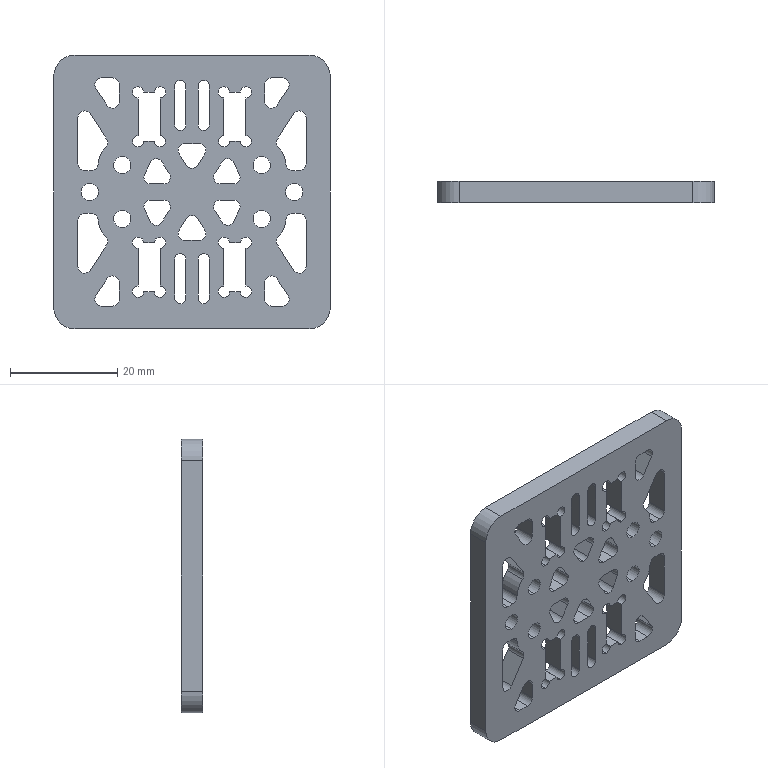Part | SolidWorks | features Fillet 2, Extrusion 1, HoleWzd 1, ICE 1 | 1 solid | 189 faces | box 51.5 x 4 x 51 mm | volume 7707 mm3 | cylinder 109 | plane 72 | cone 8 | commonest cylinder face diameters 2.5 x53 2.1 x36 3.2 x12 8 x4 9 x4